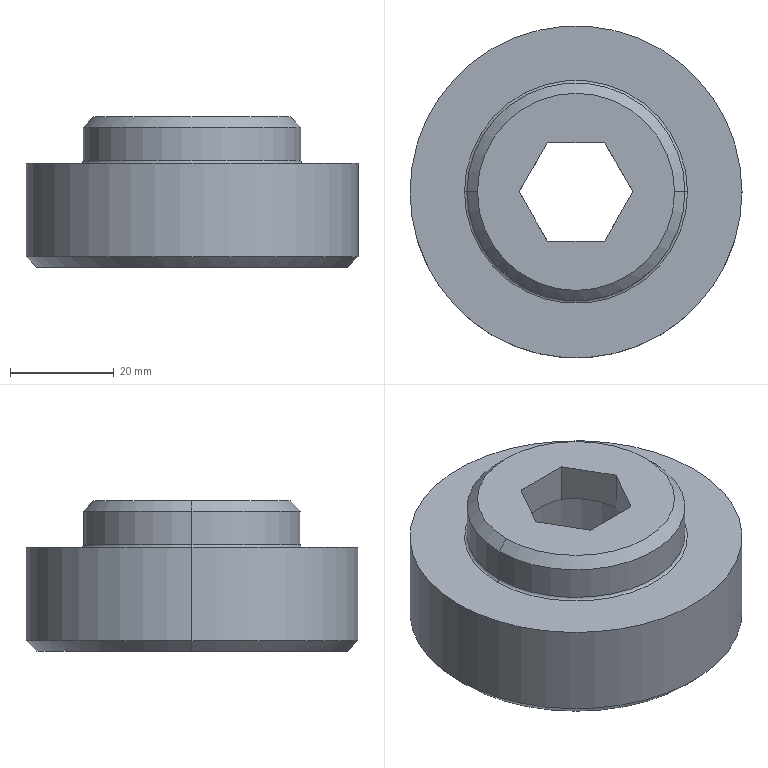Part | SolidWorks | features Chamfer 2, ICE 2, 3DProfileFeature 1, Extrusion 1, Fillet 1, HoleWzd 1 | 1 solid | 23 faces | box 64 x 64 x 29 mm | volume 46539 mm3 | plane 9 | cone 6 | cylinder 6 | torus 2 | commonest cylinder face diameters 42 x2 43 x2 64 x2
STEP:
#1=CARTESIAN_POINT('',(-21.,0.,20.5));
#2=VERTEX_POINT('',#1);
#3=CARTESIAN_POINT('',(21.,0.,20.5));
#4=VERTEX_POINT('',#3);
#5=CARTESIAN_POINT('',(0.,0.,20.5));
#6=DIRECTION('',(0.,0.,1.));
#7=DIRECTION('',(1.,0.,0.));
#8=AXIS2_PLACEMENT_3D('',#5,#6,#7);
#9=CIRCLE('',#8,21.);
#10=EDGE_CURVE('',#2,#4,#9,.T.);
#11=ORIENTED_EDGE('',*,*,#10,.F.);
#12=CARTESIAN_POINT('',(-21.5,0.,20.));
#13=VERTEX_POINT('',#12);
#14=CARTESIAN_POINT('',(-21.5,0.,20.5));
#15=DIRECTION('',(0.,1.,0.));
#16=DIRECTION('',(-1.,0.,0.));
#17=AXIS2_PLACEMENT_3D('',#14,#15,#16);
#18=CIRCLE('',#17,0.5);
#19=EDGE_CURVE('',#2,#13,#18,.T.);
#20=ORIENTED_EDGE('',*,*,#19,.T.);
#21=CARTESIAN_POINT('',(21.5,0.,20.));
#22=VERTEX_POINT('',#21);
#23=CARTESIAN_POINT('',(0.,0.,20.));
#24=DIRECTION('',(0.,0.,-1.));
#25=DIRECTION('',(1.,0.,0.));
#26=AXIS2_PLACEMENT_3D('',#23,#24,#25);
#27=CIRCLE('',#26,21.5);
#28=EDGE_CURVE('',#22,#13,#27,.T.);
#29=ORIENTED_EDGE('',*,*,#28,.F.);
#30=CARTESIAN_POINT('',(21.5,0.,20.5));
#31=DIRECTION('',(0.,-1.,0.));
#32=DIRECTION('',(0.,0.,-1.));
#33=AXIS2_PLACEMENT_3D('',#30,#31,#32);
#34=CIRCLE('',#33,0.5);
#35=EDGE_CURVE('',#4,#22,#34,.T.);
#36=ORIENTED_EDGE('',*,*,#35,.F.);
#37=EDGE_LOOP('',(#11,#20,#29,#36));
#38=FACE_OUTER_BOUND('',#37,.T.);
#39=CARTESIAN_POINT('',(0.,0.,20.5));
#40=DIRECTION('',(0.,0.,1.));
#41=DIRECTION('',(1.,0.,0.));
#42=AXIS2_PLACEMENT_3D('',#39,#40,#41);
#43=TOROIDAL_SURFACE('',#42,21.5,0.5);
#44=ADVANCED_FACE('',(#38),#43,.F.);
#45=CARTESIAN_POINT('',(19.,0.,29.));
#46=VERTEX_POINT('',#45);
#47=CARTESIAN_POINT('',(-19.,0.,29.));
#48=VERTEX_POINT('',#47);
#49=CARTESIAN_POINT('',(0.,0.,29.));
#50=DIRECTION('',(0.,0.,1.));
#51=DIRECTION('',(1.,0.,0.));
#52=AXIS2_PLACEMENT_3D('',#49,#50,#51);
#53=CIRCLE('',#52,19.);
#54=EDGE_CURVE('',#46,#48,#53,.T.);
#55=ORIENTED_EDGE('',*,*,#54,.F.);
#56=CARTESIAN_POINT('',(21.,0.,27.));
#57=VERTEX_POINT('',#56);
#58=CARTESIAN_POINT('',(19.,0.,29.));
#59=DIRECTION('',(0.7071,0.,-0.7071));
#60=VECTOR('',#59,1000.);
#61=LINE('',#58,#60);
#62=EDGE_CURVE('',#46,#57,#61,.T.);
#63=ORIENTED_EDGE('',*,*,#62,.T.);
#64=CARTESIAN_POINT('',(-21.,0.,27.));
#65=VERTEX_POINT('',#64);
#66=CARTESIAN_POINT('',(0.,0.,27.));
#67=DIRECTION('',(0.,0.,-1.));
#68=DIRECTION('',(1.,0.,0.));
#69=AXIS2_PLACEMENT_3D('',#66,#67,#68);
#70=CIRCLE('',#69,21.);
#71=EDGE_CURVE('',#65,#57,#70,.T.);
#72=ORIENTED_EDGE('',*,*,#71,.F.);
#73=CARTESIAN_POINT('',(-19.,0.,29.));
#74=DIRECTION('',(-0.7071,0.,-0.7071));
#75=VECTOR('',#74,1000.);
#76=LINE('',#73,#75);
#77=EDGE_CURVE('',#48,#65,#76,.T.);
#78=ORIENTED_EDGE('',*,*,#77,.F.);
#79=EDGE_LOOP('',(#55,#63,#72,#78));
#80=FACE_OUTER_BOUND('',#79,.T.);
#81=CARTESIAN_POINT('',(0.,0.,29.));
#82=DIRECTION('',(0.,0.,-1.));
#83=DIRECTION('',(-1.,0.,0.));
#84=AXIS2_PLACEMENT_3D('',#81,#82,#83);
#85=CONICAL_SURFACE('',#84,19.,0.7854);
#86=ADVANCED_FACE('',(#80),#85,.T.);
#87=CARTESIAN_POINT('',(-30.,0.,0.));
#88=VERTEX_POINT('',#87);
#89=CARTESIAN_POINT('',(30.,0.,0.));
#90=VERTEX_POINT('',#89);
#91=CARTESIAN_POINT('',(0.,0.,0.));
#92=DIRECTION('',(0.,0.,-1.));
#93=DIRECTION('',(1.,0.,0.));
#94=AXIS2_PLACEMENT_3D('',#91,#92,#93);
#95=CIRCLE('',#94,30.);
#96=EDGE_CURVE('',#88,#90,#95,.T.);
#97=ORIENTED_EDGE('',*,*,#96,.F.);
#98=CARTESIAN_POINT('',(-32.,0.,2.));
#99=VERTEX_POINT('',#98);
#100=CARTESIAN_POINT('',(-32.,0.,2.));
#101=DIRECTION('',(-0.7071,0.,0.7071));
#102=VECTOR('',#101,1000.);
#103=LINE('',#100,#102);
#104=EDGE_CURVE('',#88,#99,#103,.T.);
#105=ORIENTED_EDGE('',*,*,#104,.T.);
#106=CARTESIAN_POINT('',(32.,0.,2.));
#107=VERTEX_POINT('',#106);
#108=CARTESIAN_POINT('',(0.,0.,2.));
#109=DIRECTION('',(0.,0.,1.));
#110=DIRECTION('',(1.,0.,0.));
#111=AXIS2_PLACEMENT_3D('',#108,#109,#110);
#112=CIRCLE('',#111,32.);
#113=EDGE_CURVE('',#107,#99,#112,.T.);
#114=ORIENTED_EDGE('',*,*,#113,.F.);
#115=CARTESIAN_POINT('',(32.,0.,2.));
#116=DIRECTION('',(0.7071,0.,0.7071));
#117=VECTOR('',#116,1000.);
#118=LINE('',#115,#117);
#119=EDGE_CURVE('',#90,#107,#118,.T.);
#120=ORIENTED_EDGE('',*,*,#119,.F.);
#121=EDGE_LOOP('',(#97,#105,#114,#120));
#122=FACE_OUTER_BOUND('',#121,.T.);
#123=CARTESIAN_POINT('',(0.,0.,2.));
#124=DIRECTION('',(0.,0.,1.));
#125=DIRECTION('',(1.,0.,0.));
#126=AXIS2_PLACEMENT_3D('',#123,#124,#125);
#127=CONICAL_SURFACE('',#126,32.,0.7854);
#128=ADVANCED_FACE('',(#122),#127,.T.);
#129=CARTESIAN_POINT('',(21.5,0.,15.));
#130=VERTEX_POINT('',#129);
#131=CARTESIAN_POINT('',(-21.5,0.,15.));
#132=VERTEX_POINT('',#131);
#133=CARTESIAN_POINT('',(0.,0.,15.));
#134=DIRECTION('',(0.,0.,-1.));
#135=DIRECTION('',(-1.,0.,0.));
#136=AXIS2_PLACEMENT_3D('',#133,#134,#135);
#137=CIRCLE('',#136,21.5);
#138=EDGE_CURVE('',#130,#132,#137,.T.);
#139=ORIENTED_EDGE('',*,*,#138,.F.);
#140=CARTESIAN_POINT('',(21.5,0.,0.));
#141=VERTEX_POINT('',#140);
#142=CARTESIAN_POINT('',(21.5,0.,0.));
#143=DIRECTION('',(0.,0.,-1.));
#144=VECTOR('',#143,1000.);
#145=LINE('',#142,#144);
#146=EDGE_CURVE('',#130,#141,#145,.T.);
#147=ORIENTED_EDGE('',*,*,#146,.T.);
#148=CARTESIAN_POINT('',(-21.5,0.,0.));
#149=VERTEX_POINT('',#148);
#150=CARTESIAN_POINT('',(0.,0.,0.));
#151=DIRECTION('',(0.,0.,-1.));
#152=DIRECTION('',(-1.,0.,0.));
#153=AXIS2_PLACEMENT_3D('',#150,#151,#152);
#154=CIRCLE('',#153,21.5);
#155=EDGE_CURVE('',#141,#149,#154,.T.);
#156=ORIENTED_EDGE('',*,*,#155,.T.);
#157=CARTESIAN_POINT('',(-21.5,0.,0.));
#158=DIRECTION('',(0.,0.,-1.));
#159=VECTOR('',#158,1000.);
#160=LINE('',#157,#159);
#161=EDGE_CURVE('',#132,#149,#160,.T.);
#162=ORIENTED_EDGE('',*,*,#161,.F.);
#163=EDGE_LOOP('',(#139,#147,#156,#162));
#164=FACE_OUTER_BOUND('',#163,.T.);
#165=CARTESIAN_POINT('',(0.,0.,0.));
#166=DIRECTION('',(0.,0.,-1.));
#167=DIRECTION('',(-1.,0.,0.));
#168=AXIS2_PLACEMENT_3D('',#165,#166,#167);
#169=CYLINDRICAL_SURFACE('',#168,21.5);
#170=ADVANCED_FACE('',(#164),#169,.F.);
#171=CARTESIAN_POINT('',(5.485,-9.5,21.327));
#172=VERTEX_POINT('',#171);
#173=CARTESIAN_POINT('',(10.97,0.,21.327));
#174=VERTEX_POINT('',#173);
#175=CARTESIAN_POINT('',(5.485,-9.5,21.327));
#176=CARTESIAN_POINT('',(5.932,-8.726,21.596));
#177=CARTESIAN_POINT('',(6.382,-7.945,21.817));
#178=CARTESIAN_POINT('',(7.294,-6.367,22.125));
#179=CARTESIAN_POINT('',(7.754,-5.569,22.21));
#180=CARTESIAN_POINT('',(8.455,-4.356,22.211));
#181=CARTESIAN_POINT('',(8.689,-3.949,22.19));
#182=CARTESIAN_POINT('',(9.153,-3.146,22.109));
#183=CARTESIAN_POINT('',(9.384,-2.747,22.05));
#184=CARTESIAN_POINT('',(10.07,-1.558,21.819));
#185=CARTESIAN_POINT('',(10.522,-0.7754,21.596));
#186=CARTESIAN_POINT('',(10.97,0.,21.327));
#187=B_SPLINE_CURVE_WITH_KNOTS('',3,(#175,#176,#177,#178,#179,#180,#181,#182,#183,#184,#185,#186),.UNSPECIFIED.,.F.,.F.,(4,2,2,2,2,4),(0.000000239,0.002772,0.005543,0.006929,0.008315,0.01109),.UNSPECIFIED.);
#188=EDGE_CURVE('',#172,#174,#187,.T.);
#189=ORIENTED_EDGE('',*,*,#188,.T.);
#190=CARTESIAN_POINT('',(21.5,0.,15.));
#191=DIRECTION('',(0.8572,0.,-0.515));
#192=VECTOR('',#191,1000.);
#193=LINE('',#190,#192);
#194=EDGE_CURVE('',#174,#130,#193,.T.);
#195=ORIENTED_EDGE('',*,*,#194,.T.);
#196=ORIENTED_EDGE('',*,*,#138,.T.);
#197=CARTESIAN_POINT('',(-10.97,0.,21.327));
#198=VERTEX_POINT('',#197);
#199=CARTESIAN_POINT('',(-21.5,0.,15.));
#200=DIRECTION('',(-0.8572,0.,-0.515));
#201=VECTOR('',#200,1000.);
#202=LINE('',#199,#201);
#203=EDGE_CURVE('',#198,#132,#202,.T.);
#204=ORIENTED_EDGE('',*,*,#203,.F.);
#205=CARTESIAN_POINT('',(-5.485,-9.5,21.327));
#206=VERTEX_POINT('',#205);
#207=CARTESIAN_POINT('',(-10.97,0.,21.327));
#208=CARTESIAN_POINT('',(-10.523,-0.7743,21.596));
#209=CARTESIAN_POINT('',(-10.072,-1.555,21.817));
#210=CARTESIAN_POINT('',(-9.161,-3.133,22.125));
#211=CARTESIAN_POINT('',(-8.7,-3.931,22.21));
#212=CARTESIAN_POINT('',(-8.,-5.144,22.211));
#213=CARTESIAN_POINT('',(-7.765,-5.551,22.19));
#214=CARTESIAN_POINT('',(-7.301,-6.354,22.109));
#215=CARTESIAN_POINT('',(-7.071,-6.753,22.05));
#216=CARTESIAN_POINT('',(-6.384,-7.942,21.819));
#217=CARTESIAN_POINT('',(-5.933,-8.725,21.596));
#218=CARTESIAN_POINT('',(-5.485,-9.5,21.327));
#219=B_SPLINE_CURVE_WITH_KNOTS('',3,(#207,#208,#209,#210,#211,#212,#213,#214,#215,#216,#217,#218),.UNSPECIFIED.,.F.,.F.,(4,2,2,2,2,4),(0.000000239,0.002772,0.005543,0.006929,0.008315,0.01109),.UNSPECIFIED.);
#220=EDGE_CURVE('',#198,#206,#219,.T.);
#221=ORIENTED_EDGE('',*,*,#220,.T.);
#222=CARTESIAN_POINT('',(-5.485,-9.5,21.327));
#223=CARTESIAN_POINT('',(-4.596,-9.5,21.594));
#224=CARTESIAN_POINT('',(-3.69,-9.5,21.818));
#225=CARTESIAN_POINT('',(-1.842,-9.5,22.128));
#226=CARTESIAN_POINT('',(-0.919,-9.5,22.211));
#227=CARTESIAN_POINT('',(0.9268,-9.5,22.21));
#228=CARTESIAN_POINT('',(1.849,-9.5,22.128));
#229=CARTESIAN_POINT('',(3.233,-9.5,21.895));
#230=CARTESIAN_POINT('',(3.692,-9.5,21.8));
#231=CARTESIAN_POINT('',(4.596,-9.5,21.582));
#232=CARTESIAN_POINT('',(5.042,-9.5,21.46));
#233=CARTESIAN_POINT('',(5.485,-9.5,21.327));
#234=B_SPLINE_CURVE_WITH_KNOTS('',3,(#222,#223,#224,#225,#226,#227,#228,#229,#230,#231,#232,#233),.UNSPECIFIED.,.F.,.F.,(4,2,2,2,2,4),(0.01879,0.02159,0.02438,0.02717,0.02857,0.02996),.UNSPECIFIED.);
#235=EDGE_CURVE('',#206,#172,#234,.T.);
#236=ORIENTED_EDGE('',*,*,#235,.T.);
#237=EDGE_LOOP('',(#189,#195,#196,#204,#221,#236));
#238=FACE_OUTER_BOUND('',#237,.T.);
#239=CARTESIAN_POINT('',(0.,0.,15.));
#240=DIRECTION('',(0.,0.,-1.));
#241=DIRECTION('',(-1.,0.,0.));
#242=AXIS2_PLACEMENT_3D('',#239,#240,#241);
#243=CONICAL_SURFACE('',#242,21.5,1.03);
#244=ADVANCED_FACE('',(#238),#243,.F.);
#245=ORIENTED_EDGE('',*,*,#71,.T.);
#246=CARTESIAN_POINT('',(21.,0.,29.));
#247=DIRECTION('',(0.,0.,-1.));
#248=VECTOR('',#247,1000.);
#249=LINE('',#246,#248);
#250=EDGE_CURVE('',#57,#4,#249,.T.);
#251=ORIENTED_EDGE('',*,*,#250,.T.);
#252=CARTESIAN_POINT('',(0.,0.,20.5));
#253=DIRECTION('',(0.,0.,1.));
#254=DIRECTION('',(1.,0.,0.));
#255=AXIS2_PLACEMENT_3D('',#252,#253,#254);
#256=CIRCLE('',#255,21.);
#257=EDGE_CURVE('',#4,#2,#256,.T.);
#258=ORIENTED_EDGE('',*,*,#257,.T.);
#259=CARTESIAN_POINT('',(-21.,0.,29.));
#260=DIRECTION('',(0.,0.,-1.));
#261=VECTOR('',#260,1000.);
#262=LINE('',#259,#261);
#263=EDGE_CURVE('',#65,#2,#262,.T.);
#264=ORIENTED_EDGE('',*,*,#263,.F.);
#265=EDGE_LOOP('',(#245,#251,#258,#264));
#266=FACE_OUTER_BOUND('',#265,.T.);
#267=CARTESIAN_POINT('',(0.,0.,29.));
#268=DIRECTION('',(0.,0.,-1.));
#269=DIRECTION('',(-1.,0.,0.));
#270=AXIS2_PLACEMENT_3D('',#267,#268,#269);
#271=CYLINDRICAL_SURFACE('',#270,21.);
#272=ADVANCED_FACE('',(#266),#271,.T.);
#273=CARTESIAN_POINT('',(32.,0.,20.));
#274=VERTEX_POINT('',#273);
#275=CARTESIAN_POINT('',(-32.,0.,20.));
#276=VERTEX_POINT('',#275);
#277=CARTESIAN_POINT('',(0.,0.,20.));
#278=DIRECTION('',(0.,0.,1.));
#279=DIRECTION('',(1.,0.,0.));
#280=AXIS2_PLACEMENT_3D('',#277,#278,#279);
#281=CIRCLE('',#280,32.);
#282=EDGE_CURVE('',#274,#276,#281,.T.);
#283=ORIENTED_EDGE('',*,*,#282,.F.);
#284=CARTESIAN_POINT('',(32.,0.,20.));
#285=DIRECTION('',(0.,0.,-1.));
#286=VECTOR('',#285,1000.);
#287=LINE('',#284,#286);
#288=EDGE_CURVE('',#274,#107,#287,.T.);
#289=ORIENTED_EDGE('',*,*,#288,.T.);
#290=ORIENTED_EDGE('',*,*,#113,.T.);
#291=CARTESIAN_POINT('',(-32.,0.,20.));
#292=DIRECTION('',(0.,0.,-1.));
#293=VECTOR('',#292,1000.);
#294=LINE('',#291,#293);
#295=EDGE_CURVE('',#276,#99,#294,.T.);
#296=ORIENTED_EDGE('',*,*,#295,.F.);
#297=EDGE_LOOP('',(#283,#289,#290,#296));
#298=FACE_OUTER_BOUND('',#297,.T.);
#299=CARTESIAN_POINT('',(0.,0.,20.));
#300=DIRECTION('',(0.,0.,-1.));
#301=DIRECTION('',(-1.,0.,0.));
#302=AXIS2_PLACEMENT_3D('',#299,#300,#301);
#303=CYLINDRICAL_SURFACE('',#302,32.);
#304=ADVANCED_FACE('',(#298),#303,.T.);
#305=ORIENTED_EDGE('',*,*,#288,.F.);
#306=CARTESIAN_POINT('',(0.,0.,20.));
#307=DIRECTION('',(0.,0.,1.));
#308=DIRECTION('',(1.,0.,0.));
#309=AXIS2_PLACEMENT_3D('',#306,#307,#308);
#310=CIRCLE('',#309,32.);
#311=EDGE_CURVE('',#276,#274,#310,.T.);
#312=ORIENTED_EDGE('',*,*,#311,.F.);
#313=ORIENTED_EDGE('',*,*,#295,.T.);
#314=CARTESIAN_POINT('',(0.,0.,2.));
#315=DIRECTION('',(0.,0.,1.));
#316=DIRECTION('',(1.,0.,0.));
#317=AXIS2_PLACEMENT_3D('',#314,#315,#316);
#318=CIRCLE('',#317,32.);
#319=EDGE_CURVE('',#99,#107,#318,.T.);
#320=ORIENTED_EDGE('',*,*,#319,.T.);
#321=EDGE_LOOP('',(#305,#312,#313,#320));
#322=FACE_OUTER_BOUND('',#321,.T.);
#323=CARTESIAN_POINT('',(0.,0.,20.));
#324=DIRECTION('',(0.,0.,-1.));
#325=DIRECTION('',(-1.,0.,0.));
#326=AXIS2_PLACEMENT_3D('',#323,#324,#325);
#327=CYLINDRICAL_SURFACE('',#326,32.);
#328=ADVANCED_FACE('',(#322),#327,.T.);
#329=ORIENTED_EDGE('',*,*,#28,.T.);
#330=CARTESIAN_POINT('',(0.,0.,20.));
#331=DIRECTION('',(0.,0.,-1.));
#332=DIRECTION('',(1.,0.,0.));
#333=AXIS2_PLACEMENT_3D('',#330,#331,#332);
#334=CIRCLE('',#333,21.5);
#335=EDGE_CURVE('',#13,#22,#334,.T.);
#336=ORIENTED_EDGE('',*,*,#335,.T.);
#337=EDGE_LOOP('',(#329,#336));
#338=FACE_BOUND('',#337,.T.);
#339=ORIENTED_EDGE('',*,*,#311,.T.);
#340=ORIENTED_EDGE('',*,*,#282,.T.);
#341=EDGE_LOOP('',(#339,#340));
#342=FACE_OUTER_BOUND('',#341,.T.);
#343=CARTESIAN_POINT('',(0.,0.,20.));
#344=DIRECTION('',(0.,0.,1.));
#345=DIRECTION('',(1.,0.,0.));
#346=AXIS2_PLACEMENT_3D('',#343,#344,#345);
#347=PLANE('',#346);
#348=ADVANCED_FACE('',(#338,#342),#347,.T.);
#349=CARTESIAN_POINT('',(0.,0.,0.));
#350=DIRECTION('',(0.,0.,-1.));
#351=DIRECTION('',(1.,0.,0.));
#352=AXIS2_PLACEMENT_3D('',#349,#350,#351);
#353=CIRCLE('',#352,30.);
#354=EDGE_CURVE('',#90,#88,#353,.T.);
#355=ORIENTED_EDGE('',*,*,#354,.T.);
#356=ORIENTED_EDGE('',*,*,#96,.T.);
#357=EDGE_LOOP('',(#355,#356));
#358=FACE_OUTER_BOUND('',#357,.T.);
#359=CARTESIAN_POINT('',(0.,0.,0.));
#360=DIRECTION('',(0.,0.,-1.));
#361=DIRECTION('',(-1.,0.,0.));
#362=AXIS2_PLACEMENT_3D('',#359,#360,#361);
#363=CIRCLE('',#362,21.5);
#364=EDGE_CURVE('',#149,#141,#363,.T.);
#365=ORIENTED_EDGE('',*,*,#364,.F.);
#366=ORIENTED_EDGE('',*,*,#155,.F.);
#367=EDGE_LOOP('',(#365,#366));
#368=FACE_BOUND('',#367,.T.);
#369=CARTESIAN_POINT('',(0.,0.,0.));
#370=DIRECTION('',(0.,0.,1.));
#371=DIRECTION('',(1.,0.,0.));
#372=AXIS2_PLACEMENT_3D('',#369,#370,#371);
#373=PLANE('',#372);
#374=ADVANCED_FACE('',(#358,#368),#373,.F.);
#375=ORIENTED_EDGE('',*,*,#250,.F.);
#376=CARTESIAN_POINT('',(0.,0.,27.));
#377=DIRECTION('',(0.,0.,-1.));
#378=DIRECTION('',(1.,0.,0.));
#379=AXIS2_PLACEMENT_3D('',#376,#377,#378);
#380=CIRCLE('',#379,21.);
#381=EDGE_CURVE('',#57,#65,#380,.T.);
#382=ORIENTED_EDGE('',*,*,#381,.T.);
#383=ORIENTED_EDGE('',*,*,#263,.T.);
#384=ORIENTED_EDGE('',*,*,#10,.T.);
#385=EDGE_LOOP('',(#375,#382,#383,#384));
#386=FACE_OUTER_BOUND('',#385,.T.);
#387=CARTESIAN_POINT('',(0.,0.,29.));
#388=DIRECTION('',(0.,0.,-1.));
#389=DIRECTION('',(-1.,0.,0.));
#390=AXIS2_PLACEMENT_3D('',#387,#388,#389);
#391=CYLINDRICAL_SURFACE('',#390,21.);
#392=ADVANCED_FACE('',(#386),#391,.T.);
#393=CARTESIAN_POINT('',(0.,0.,29.));
#394=DIRECTION('',(0.,0.,1.));
#395=DIRECTION('',(1.,0.,0.));
#396=AXIS2_PLACEMENT_3D('',#393,#394,#395);
#397=CIRCLE('',#396,19.);
#398=EDGE_CURVE('',#48,#46,#397,.T.);
#399=ORIENTED_EDGE('',*,*,#398,.T.);
#400=ORIENTED_EDGE('',*,*,#54,.T.);
#401=EDGE_LOOP('',(#399,#400));
#402=FACE_OUTER_BOUND('',#401,.T.);
#403=CARTESIAN_POINT('',(5.485,-9.5,29.));
#404=VERTEX_POINT('',#403);
#405=CARTESIAN_POINT('',(10.97,0.,29.));
#406=VERTEX_POINT('',#405);
#407=CARTESIAN_POINT('',(5.485,-9.5,29.));
#408=DIRECTION('',(0.5,0.866,0.));
#409=VECTOR('',#408,1000.);
#410=LINE('',#407,#409);
#411=EDGE_CURVE('',#404,#406,#410,.T.);
#412=ORIENTED_EDGE('',*,*,#411,.F.);
#413=CARTESIAN_POINT('',(-5.485,-9.5,29.));
#414=VERTEX_POINT('',#413);
#415=CARTESIAN_POINT('',(-5.485,-9.5,29.));
#416=DIRECTION('',(1.,0.,0.));
#417=VECTOR('',#416,1000.);
#418=LINE('',#415,#417);
#419=EDGE_CURVE('',#414,#404,#418,.T.);
#420=ORIENTED_EDGE('',*,*,#419,.F.);
#421=CARTESIAN_POINT('',(-10.97,0.,29.));
#422=VERTEX_POINT('',#421);
#423=CARTESIAN_POINT('',(-10.97,0.,29.));
#424=DIRECTION('',(0.5,-0.866,0.));
#425=VECTOR('',#424,1000.);
#426=LINE('',#423,#425);
#427=EDGE_CURVE('',#422,#414,#426,.T.);
#428=ORIENTED_EDGE('',*,*,#427,.F.);
#429=CARTESIAN_POINT('',(-5.485,9.5,29.));
#430=VERTEX_POINT('',#429);
#431=CARTESIAN_POINT('',(-5.485,9.5,29.));
#432=DIRECTION('',(-0.5,-0.866,0.));
#433=VECTOR('',#432,1000.);
#434=LINE('',#431,#433);
#435=EDGE_CURVE('',#430,#422,#434,.T.);
#436=ORIENTED_EDGE('',*,*,#435,.F.);
#437=CARTESIAN_POINT('',(5.485,9.5,29.));
#438=VERTEX_POINT('',#437);
#439=CARTESIAN_POINT('',(5.485,9.5,29.));
#440=DIRECTION('',(-1.,0.,0.));
#441=VECTOR('',#440,1000.);
#442=LINE('',#439,#441);
#443=EDGE_CURVE('',#438,#430,#442,.T.);
#444=ORIENTED_EDGE('',*,*,#443,.F.);
#445=CARTESIAN_POINT('',(10.97,0.,29.));
#446=DIRECTION('',(-0.5,0.866,0.));
#447=VECTOR('',#446,1000.);
#448=LINE('',#445,#447);
#449=EDGE_CURVE('',#406,#438,#448,.T.);
#450=ORIENTED_EDGE('',*,*,#449,.F.);
#451=EDGE_LOOP('',(#412,#420,#428,#436,#444,#450));
#452=FACE_BOUND('',#451,.T.);
#453=CARTESIAN_POINT('',(0.,0.,29.));
#454=DIRECTION('',(0.,0.,1.));
#455=DIRECTION('',(1.,0.,0.));
#456=AXIS2_PLACEMENT_3D('',#453,#454,#455);
#457=PLANE('',#456);
#458=ADVANCED_FACE('',(#402,#452),#457,.T.);
#459=ORIENTED_EDGE('',*,*,#194,.F.);
#460=CARTESIAN_POINT('',(5.485,9.5,21.327));
#461=VERTEX_POINT('',#460);
#462=CARTESIAN_POINT('',(10.97,0.,21.327));
#463=CARTESIAN_POINT('',(10.523,0.7743,21.596));
#464=CARTESIAN_POINT('',(10.072,1.555,21.817));
#465=CARTESIAN_POINT('',(9.161,3.133,22.125));
#466=CARTESIAN_POINT('',(8.7,3.931,22.21));
#467=CARTESIAN_POINT('',(8.,5.144,22.211));
#468=CARTESIAN_POINT('',(7.765,5.551,22.19));
#469=CARTESIAN_POINT('',(7.301,6.354,22.109));
#470=CARTESIAN_POINT('',(7.071,6.753,22.05));
#471=CARTESIAN_POINT('',(6.384,7.942,21.819));
#472=CARTESIAN_POINT('',(5.933,8.725,21.596));
#473=CARTESIAN_POINT('',(5.485,9.5,21.327));
#474=B_SPLINE_CURVE_WITH_KNOTS('',3,(#462,#463,#464,#465,#466,#467,#468,#469,#470,#471,#472,#473),.UNSPECIFIED.,.F.,.F.,(4,2,2,2,2,4),(0.000000239,0.002772,0.005543,0.006929,0.008315,0.01109),.UNSPECIFIED.);
#475=EDGE_CURVE('',#174,#461,#474,.T.);
#476=ORIENTED_EDGE('',*,*,#475,.T.);
#477=CARTESIAN_POINT('',(-5.485,9.5,21.327));
#478=VERTEX_POINT('',#477);
#479=CARTESIAN_POINT('',(5.485,9.5,21.327));
#480=CARTESIAN_POINT('',(4.596,9.5,21.594));
#481=CARTESIAN_POINT('',(3.69,9.5,21.818));
#482=CARTESIAN_POINT('',(1.842,9.5,22.128));
#483=CARTESIAN_POINT('',(0.919,9.5,22.211));
#484=CARTESIAN_POINT('',(-0.9268,9.5,22.21));
#485=CARTESIAN_POINT('',(-1.849,9.5,22.128));
#486=CARTESIAN_POINT('',(-3.233,9.5,21.895));
#487=CARTESIAN_POINT('',(-3.692,9.5,21.8));
#488=CARTESIAN_POINT('',(-4.596,9.5,21.582));
#489=CARTESIAN_POINT('',(-5.042,9.5,21.46));
#490=CARTESIAN_POINT('',(-5.485,9.5,21.327));
#491=B_SPLINE_CURVE_WITH_KNOTS('',3,(#479,#480,#481,#482,#483,#484,#485,#486,#487,#488,#489,#490),.UNSPECIFIED.,.F.,.F.,(4,2,2,2,2,4),(0.01879,0.02159,0.02438,0.02717,0.02857,0.02996),.UNSPECIFIED.);
#492=EDGE_CURVE('',#461,#478,#491,.T.);
#493=ORIENTED_EDGE('',*,*,#492,.T.);
#494=CARTESIAN_POINT('',(-5.485,9.5,21.327));
#495=CARTESIAN_POINT('',(-5.932,8.726,21.596));
#496=CARTESIAN_POINT('',(-6.382,7.945,21.817));
#497=CARTESIAN_POINT('',(-7.294,6.367,22.125));
#498=CARTESIAN_POINT('',(-7.754,5.569,22.21));
#499=CARTESIAN_POINT('',(-8.455,4.356,22.211));
#500=CARTESIAN_POINT('',(-8.689,3.949,22.19));
#501=CARTESIAN_POINT('',(-9.153,3.146,22.109));
#502=CARTESIAN_POINT('',(-9.384,2.747,22.05));
#503=CARTESIAN_POINT('',(-10.07,1.558,21.819));
#504=CARTESIAN_POINT('',(-10.522,0.7754,21.596));
#505=CARTESIAN_POINT('',(-10.97,0.,21.327));
#506=B_SPLINE_CURVE_WITH_KNOTS('',3,(#494,#495,#496,#497,#498,#499,#500,#501,#502,#503,#504,#505),.UNSPECIFIED.,.F.,.F.,(4,2,2,2,2,4),(0.000000239,0.002772,0.005543,0.006929,0.008315,0.01109),.UNSPECIFIED.);
#507=EDGE_CURVE('',#478,#198,#506,.T.);
#508=ORIENTED_EDGE('',*,*,#507,.T.);
#509=ORIENTED_EDGE('',*,*,#203,.T.);
#510=CARTESIAN_POINT('',(0.,0.,15.));
#511=DIRECTION('',(0.,0.,-1.));
#512=DIRECTION('',(-1.,0.,0.));
#513=AXIS2_PLACEMENT_3D('',#510,#511,#512);
#514=CIRCLE('',#513,21.5);
#515=EDGE_CURVE('',#132,#130,#514,.T.);
#516=ORIENTED_EDGE('',*,*,#515,.T.);
#517=EDGE_LOOP('',(#459,#476,#493,#508,#509,#516));
#518=FACE_OUTER_BOUND('',#517,.T.);
#519=CARTESIAN_POINT('',(0.,0.,15.));
#520=DIRECTION('',(0.,0.,-1.));
#521=DIRECTION('',(-1.,0.,0.));
#522=AXIS2_PLACEMENT_3D('',#519,#520,#521);
#523=CONICAL_SURFACE('',#522,21.5,1.03);
#524=ADVANCED_FACE('',(#518),#523,.F.);
#525=ORIENTED_EDGE('',*,*,#146,.F.);
#526=ORIENTED_EDGE('',*,*,#515,.F.);
#527=ORIENTED_EDGE('',*,*,#161,.T.);
#528=ORIENTED_EDGE('',*,*,#364,.T.);
#529=EDGE_LOOP('',(#525,#526,#527,#528));
#530=FACE_OUTER_BOUND('',#529,.T.);
#531=CARTESIAN_POINT('',(0.,0.,0.));
#532=DIRECTION('',(0.,0.,-1.));
#533=DIRECTION('',(-1.,0.,0.));
#534=AXIS2_PLACEMENT_3D('',#531,#532,#533);
#535=CYLINDRICAL_SURFACE('',#534,21.5);
#536=ADVANCED_FACE('',(#530),#535,.F.);
#537=CARTESIAN_POINT('',(5.485,-9.5,0.));
#538=DIRECTION('',(0.,0.,1.));
#539=VECTOR('',#538,1000.);
#540=LINE('',#537,#539);
#541=EDGE_CURVE('',#172,#404,#540,.T.);
#542=ORIENTED_EDGE('',*,*,#541,.T.);
#543=ORIENTED_EDGE('',*,*,#411,.T.);
#544=CARTESIAN_POINT('',(10.97,0.,0.));
#545=DIRECTION('',(0.,0.,1.));
#546=VECTOR('',#545,1000.);
#547=LINE('',#544,#546);
#548=EDGE_CURVE('',#174,#406,#547,.T.);
#549=ORIENTED_EDGE('',*,*,#548,.F.);
#550=ORIENTED_EDGE('',*,*,#188,.F.);
#551=EDGE_LOOP('',(#542,#543,#549,#550));
#552=FACE_OUTER_BOUND('',#551,.T.);
#553=CARTESIAN_POINT('',(5.485,-9.5,0.));
#554=DIRECTION('',(0.866,-0.5,0.));
#555=DIRECTION('',(0.5,0.866,0.));
#556=AXIS2_PLACEMENT_3D('',#553,#554,#555);
#557=PLANE('',#556);
#558=ADVANCED_FACE('',(#552),#557,.F.);
#559=CARTESIAN_POINT('',(-5.485,-9.5,0.));
#560=DIRECTION('',(0.,0.,1.));
#561=VECTOR('',#560,1000.);
#562=LINE('',#559,#561);
#563=EDGE_CURVE('',#206,#414,#562,.T.);
#564=ORIENTED_EDGE('',*,*,#563,.T.);
#565=ORIENTED_EDGE('',*,*,#419,.T.);
#566=ORIENTED_EDGE('',*,*,#541,.F.);
#567=ORIENTED_EDGE('',*,*,#235,.F.);
#568=EDGE_LOOP('',(#564,#565,#566,#567));
#569=FACE_OUTER_BOUND('',#568,.T.);
#570=CARTESIAN_POINT('',(-5.485,-9.5,0.));
#571=DIRECTION('',(0.,-1.,0.));
#572=DIRECTION('',(1.,0.,0.));
#573=AXIS2_PLACEMENT_3D('',#570,#571,#572);
#574=PLANE('',#573);
#575=ADVANCED_FACE('',(#569),#574,.F.);
#576=CARTESIAN_POINT('',(-10.97,0.,0.));
#577=DIRECTION('',(0.,0.,1.));
#578=VECTOR('',#577,1000.);
#579=LINE('',#576,#578);
#580=EDGE_CURVE('',#198,#422,#579,.T.);
#581=ORIENTED_EDGE('',*,*,#580,.T.);
#582=ORIENTED_EDGE('',*,*,#427,.T.);
#583=ORIENTED_EDGE('',*,*,#563,.F.);
#584=ORIENTED_EDGE('',*,*,#220,.F.);
#585=EDGE_LOOP('',(#581,#582,#583,#584));
#586=FACE_OUTER_BOUND('',#585,.T.);
#587=CARTESIAN_POINT('',(-10.97,0.,0.));
#588=DIRECTION('',(-0.866,-0.5,0.));
#589=DIRECTION('',(0.5,-0.866,0.));
#590=AXIS2_PLACEMENT_3D('',#587,#588,#589);
#591=PLANE('',#590);
#592=ADVANCED_FACE('',(#586),#591,.F.);
#593=CARTESIAN_POINT('',(-5.485,9.5,0.));
#594=DIRECTION('',(0.,0.,1.));
#595=VECTOR('',#594,1000.);
#596=LINE('',#593,#595);
#597=EDGE_CURVE('',#478,#430,#596,.T.);
#598=ORIENTED_EDGE('',*,*,#597,.T.);
#599=ORIENTED_EDGE('',*,*,#435,.T.);
#600=ORIENTED_EDGE('',*,*,#580,.F.);
#601=ORIENTED_EDGE('',*,*,#507,.F.);
#602=EDGE_LOOP('',(#598,#599,#600,#601));
#603=FACE_OUTER_BOUND('',#602,.T.);
#604=CARTESIAN_POINT('',(-5.485,9.5,0.));
#605=DIRECTION('',(-0.866,0.5,0.));
#606=DIRECTION('',(-0.5,-0.866,0.));
#607=AXIS2_PLACEMENT_3D('',#604,#605,#606);
#608=PLANE('',#607);
#609=ADVANCED_FACE('',(#603),#608,.F.);
#610=CARTESIAN_POINT('',(5.485,9.5,0.));
#611=DIRECTION('',(0.,0.,1.));
#612=VECTOR('',#611,1000.);
#613=LINE('',#610,#612);
#614=EDGE_CURVE('',#461,#438,#613,.T.);
#615=ORIENTED_EDGE('',*,*,#614,.T.);
#616=ORIENTED_EDGE('',*,*,#443,.T.);
#617=ORIENTED_EDGE('',*,*,#597,.F.);
#618=ORIENTED_EDGE('',*,*,#492,.F.);
#619=EDGE_LOOP('',(#615,#616,#617,#618));
#620=FACE_OUTER_BOUND('',#619,.T.);
#621=CARTESIAN_POINT('',(5.485,9.5,0.));
#622=DIRECTION('',(0.,1.,0.));
#623=DIRECTION('',(0.,0.,1.));
#624=AXIS2_PLACEMENT_3D('',#621,#622,#623);
#625=PLANE('',#624);
#626=ADVANCED_FACE('',(#620),#625,.F.);
#627=ORIENTED_EDGE('',*,*,#548,.T.);
#628=ORIENTED_EDGE('',*,*,#449,.T.);
#629=ORIENTED_EDGE('',*,*,#614,.F.);
#630=ORIENTED_EDGE('',*,*,#475,.F.);
#631=EDGE_LOOP('',(#627,#628,#629,#630));
#632=FACE_OUTER_BOUND('',#631,.T.);
#633=CARTESIAN_POINT('',(10.97,0.,0.));
#634=DIRECTION('',(0.866,0.5,0.));
#635=DIRECTION('',(-0.5,0.866,0.));
#636=AXIS2_PLACEMENT_3D('',#633,#634,#635);
#637=PLANE('',#636);
#638=ADVANCED_FACE('',(#632),#637,.F.);
#639=ORIENTED_EDGE('',*,*,#104,.F.);
#640=ORIENTED_EDGE('',*,*,#354,.F.);
#641=ORIENTED_EDGE('',*,*,#119,.T.);
#642=ORIENTED_EDGE('',*,*,#319,.F.);
#643=EDGE_LOOP('',(#639,#640,#641,#642));
#644=FACE_OUTER_BOUND('',#643,.T.);
#645=CARTESIAN_POINT('',(0.,0.,2.));
#646=DIRECTION('',(0.,0.,1.));
#647=DIRECTION('',(1.,0.,0.));
#648=AXIS2_PLACEMENT_3D('',#645,#646,#647);
#649=CONICAL_SURFACE('',#648,32.,0.7854);
#650=ADVANCED_FACE('',(#644),#649,.T.);
#651=ORIENTED_EDGE('',*,*,#62,.F.);
#652=ORIENTED_EDGE('',*,*,#398,.F.);
#653=ORIENTED_EDGE('',*,*,#77,.T.);
#654=ORIENTED_EDGE('',*,*,#381,.F.);
#655=EDGE_LOOP('',(#651,#652,#653,#654));
#656=FACE_OUTER_BOUND('',#655,.T.);
#657=CARTESIAN_POINT('',(0.,0.,29.));
#658=DIRECTION('',(0.,0.,-1.));
#659=DIRECTION('',(-1.,0.,0.));
#660=AXIS2_PLACEMENT_3D('',#657,#658,#659);
#661=CONICAL_SURFACE('',#660,19.,0.7854);
#662=ADVANCED_FACE('',(#656),#661,.T.);
#663=ORIENTED_EDGE('',*,*,#19,.F.);
#664=ORIENTED_EDGE('',*,*,#257,.F.);
#665=ORIENTED_EDGE('',*,*,#35,.T.);
#666=ORIENTED_EDGE('',*,*,#335,.F.);
#667=EDGE_LOOP('',(#663,#664,#665,#666));
#668=FACE_OUTER_BOUND('',#667,.T.);
#669=CARTESIAN_POINT('',(0.,0.,20.5));
#670=DIRECTION('',(0.,0.,1.));
#671=DIRECTION('',(1.,0.,0.));
#672=AXIS2_PLACEMENT_3D('',#669,#670,#671);
#673=TOROIDAL_SURFACE('',#672,21.5,0.5);
#674=ADVANCED_FACE('',(#668),#673,.F.);
#675=CLOSED_SHELL('',(#44,#86,#128,#170,#244,#272,#304,#328,#348,#374,#392,#458,#524,#536,#558,#575,#592,#609,#626,#638,#650,#662,#674));
#676=MANIFOLD_SOLID_BREP('',#675);
#677=CARTESIAN_POINT('',(0.,0.,0.));
#678=DIRECTION('',(0.,0.,1.));
#679=DIRECTION('',(1.,0.,0.));
#680=AXIS2_PLACEMENT_3D('',#677,#678,#679);
#681=(LENGTH_UNIT()NAMED_UNIT(*)SI_UNIT(.MILLI.,.METRE.));
#682=UNCERTAINTY_MEASURE_WITH_UNIT(LENGTH_MEASURE(0.00001),#681,'','');
#683=(NAMED_UNIT(*)PLANE_ANGLE_UNIT()SI_UNIT($,.RADIAN.));
#684=(NAMED_UNIT(*)SI_UNIT($,.STERADIAN.)SOLID_ANGLE_UNIT());
#685=(GEOMETRIC_REPRESENTATION_CONTEXT(3)GLOBAL_UNCERTAINTY_ASSIGNED_CONTEXT((#682))GLOBAL_UNIT_ASSIGNED_CONTEXT((#681,#683,#684))REPRESENTATION_CONTEXT('',''));
#686=ADVANCED_BREP_SHAPE_REPRESENTATION('',(#676,#680),#685);